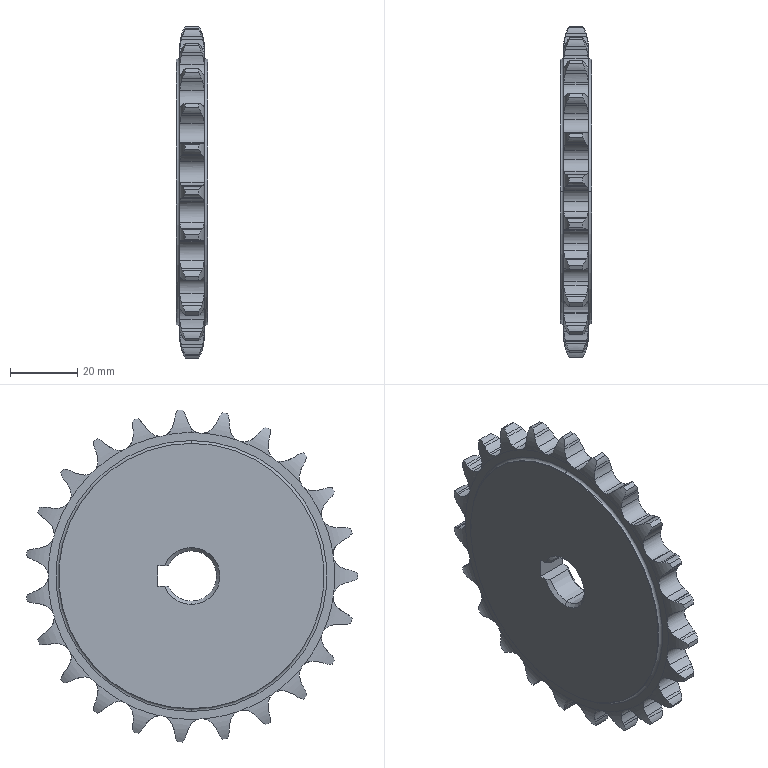Part | SolidWorks | features Chamfer 3, Cut 2, Revolution 2, CirPattern 1 | 1 solid | 268 faces | box 9.37 x 98.633 x 98.858 mm | volume 54827 mm3 | cylinder 157 | plane 53 | torus 52 | cone 6 | commonest cylinder face diameters 11.437 x49 20.732 x48 8.06 x30 99 x23 79 x4 15 x3